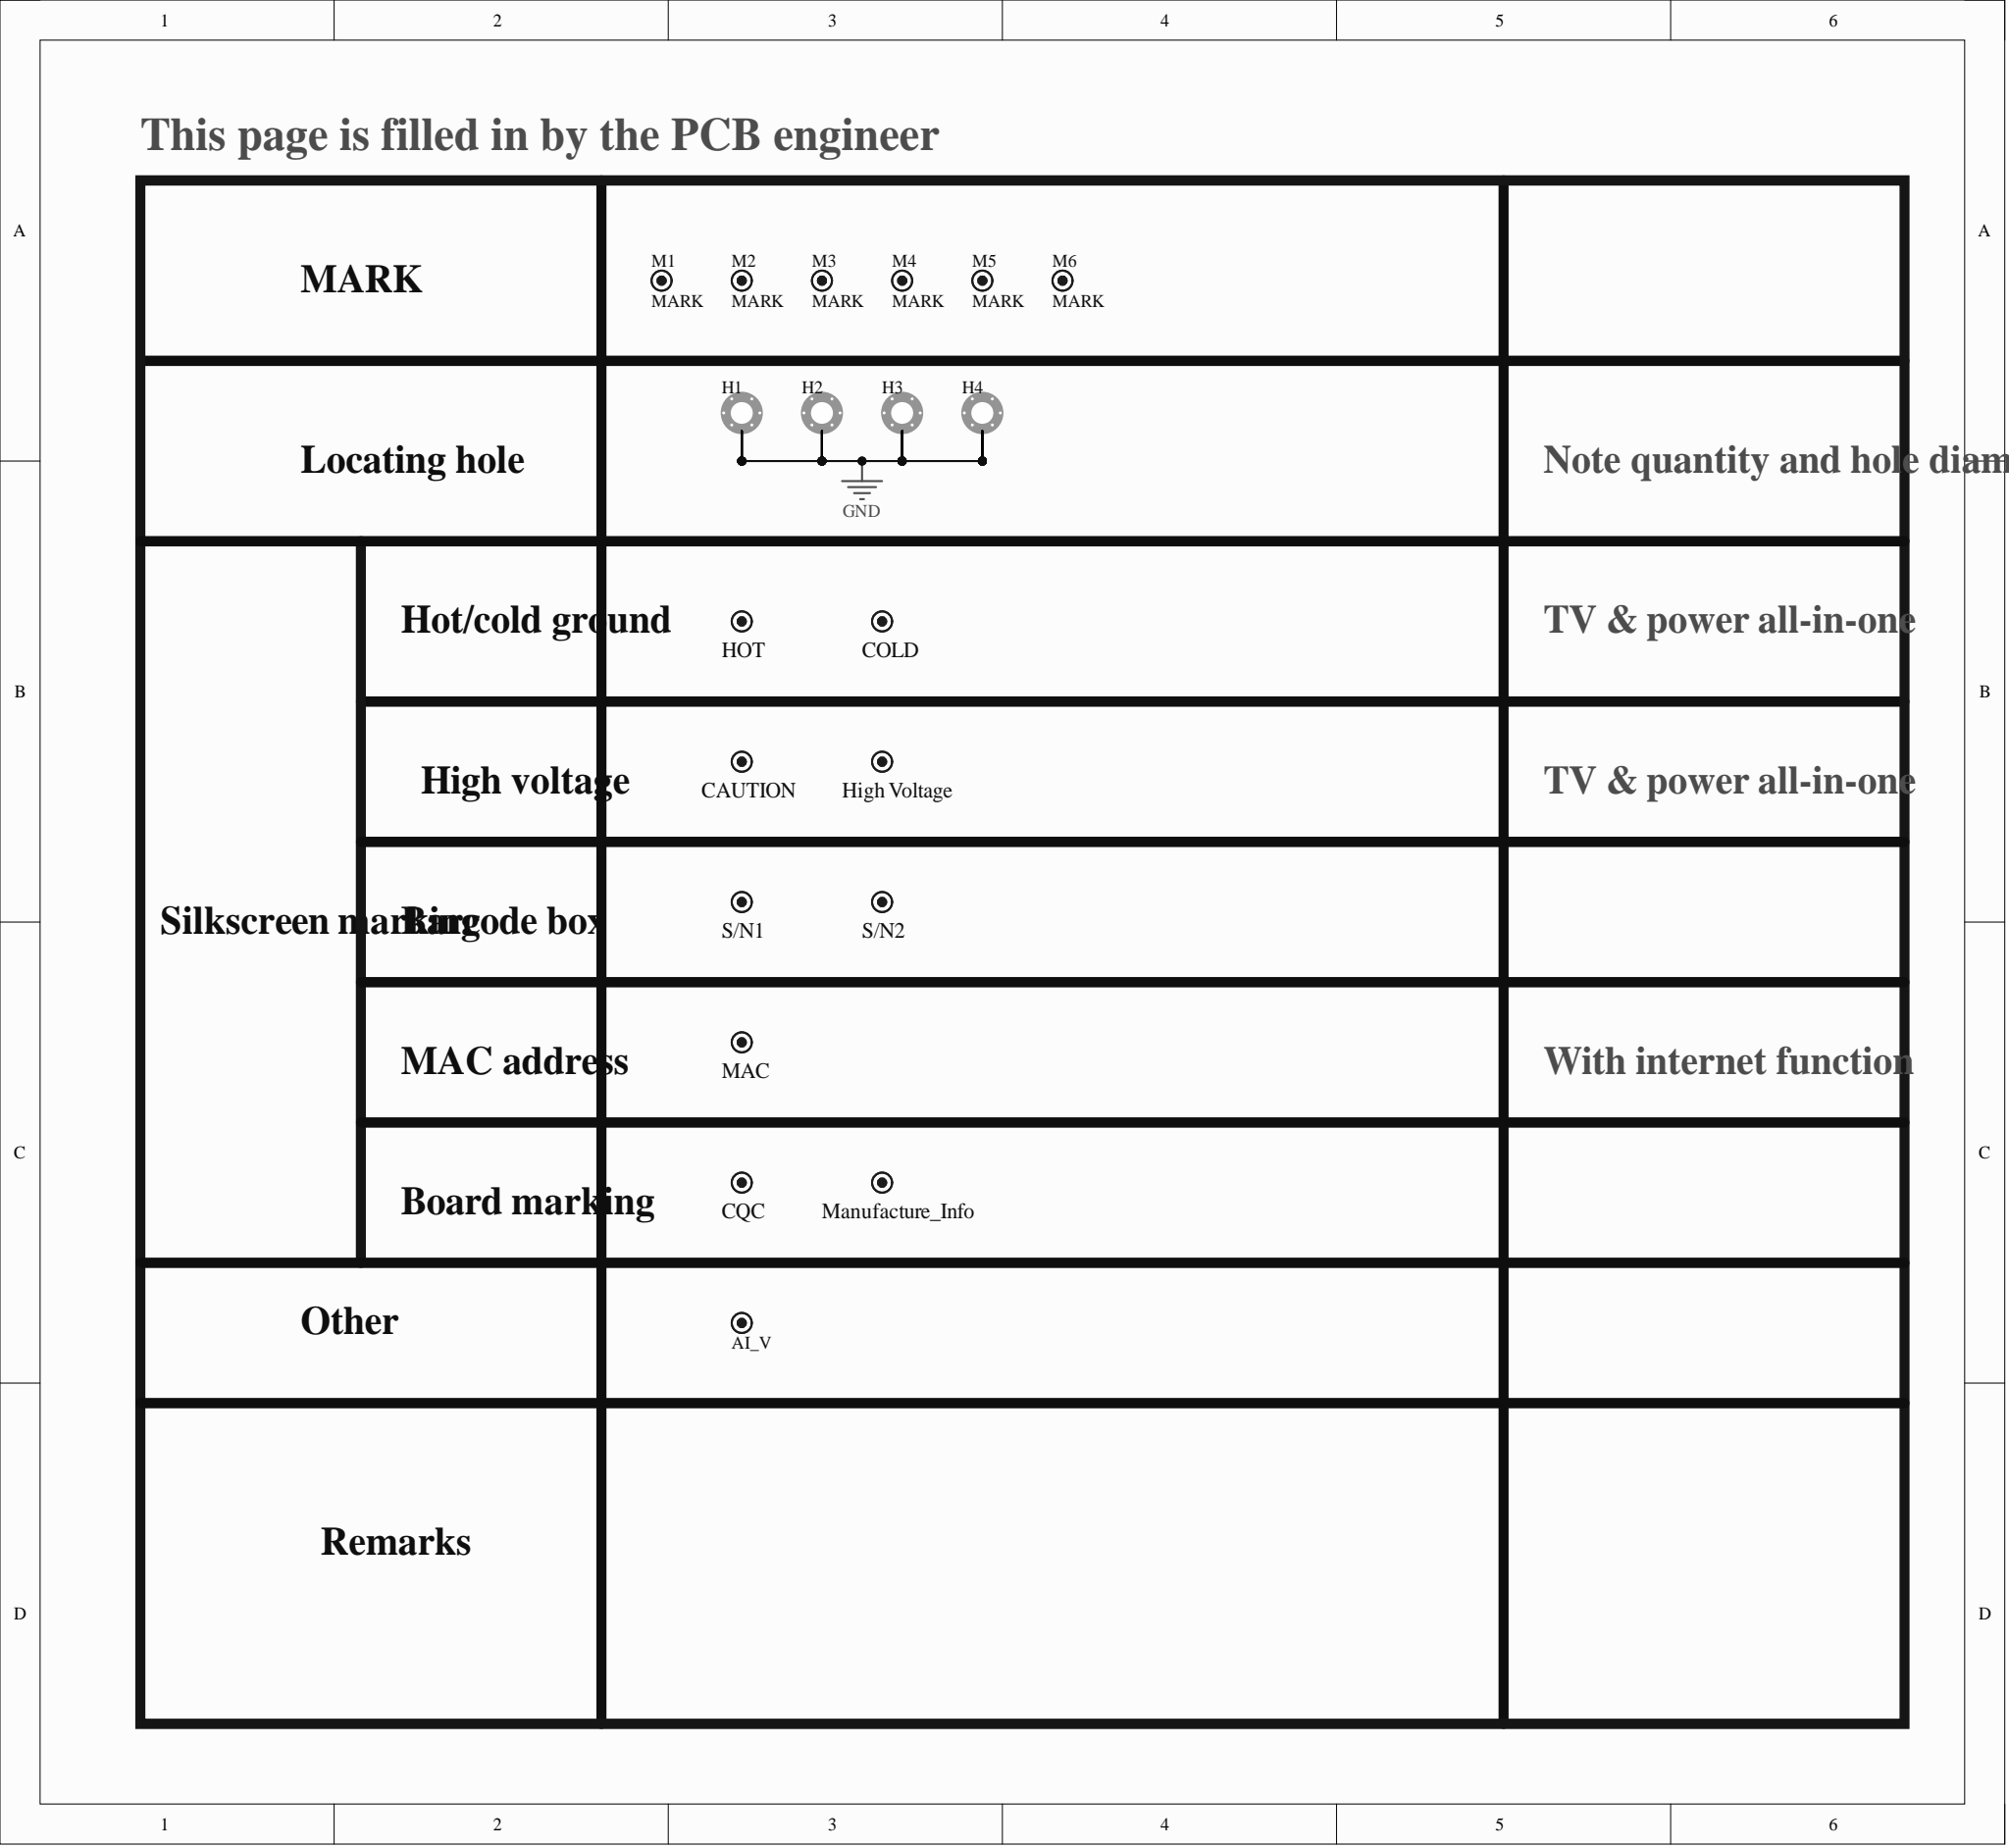Circuit board | Altium Designer | 951 parts | 509 nets | one sheet of the schematic
Parts on this sheet (reference | value | footprint):
AI_V | AI_GRIPPER_V | AI_GRIPPER_V
CAUTION | CAUTION | CAUTION
COLD | COLD | COLD
CQC | CQC | CQC
HOT | HOT | HOT
M1 | MARK | MARK
M2 | MARK | MARK
M3 | MARK | MARK
M4 | MARK | MARK
M5 | MARK | MARK
M6 | MARK | MARK
MAC | MAC | Barcode
Manufacture_Info | Manufacture_Info | Manufacture_Info
S/N1 | Barcode | Barcode
S/N2 | Barcode | Barcode
Nets of these parts (net: part-pin ...):